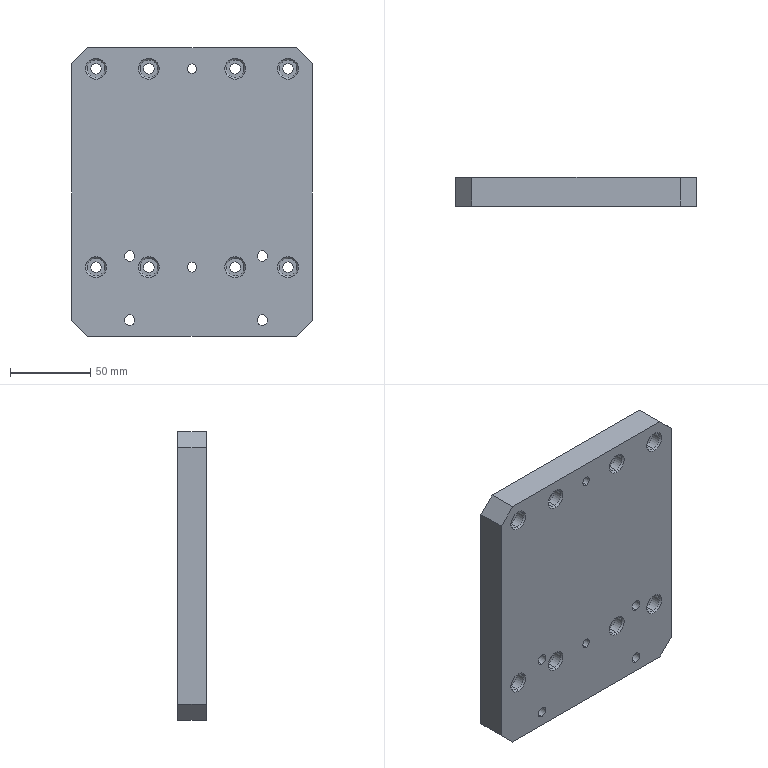Part | SolidWorks | features HoleWzd 2, Chamfer 1, Cut 1, Extrusion 1 | 1 solid | 98 faces | box 150 x 18 x 180 mm | volume 468816 mm3 | cylinder 52 | cone 24 | plane 22 | commonest cylinder face diameters 6.6 x24 11 x24 6 x4